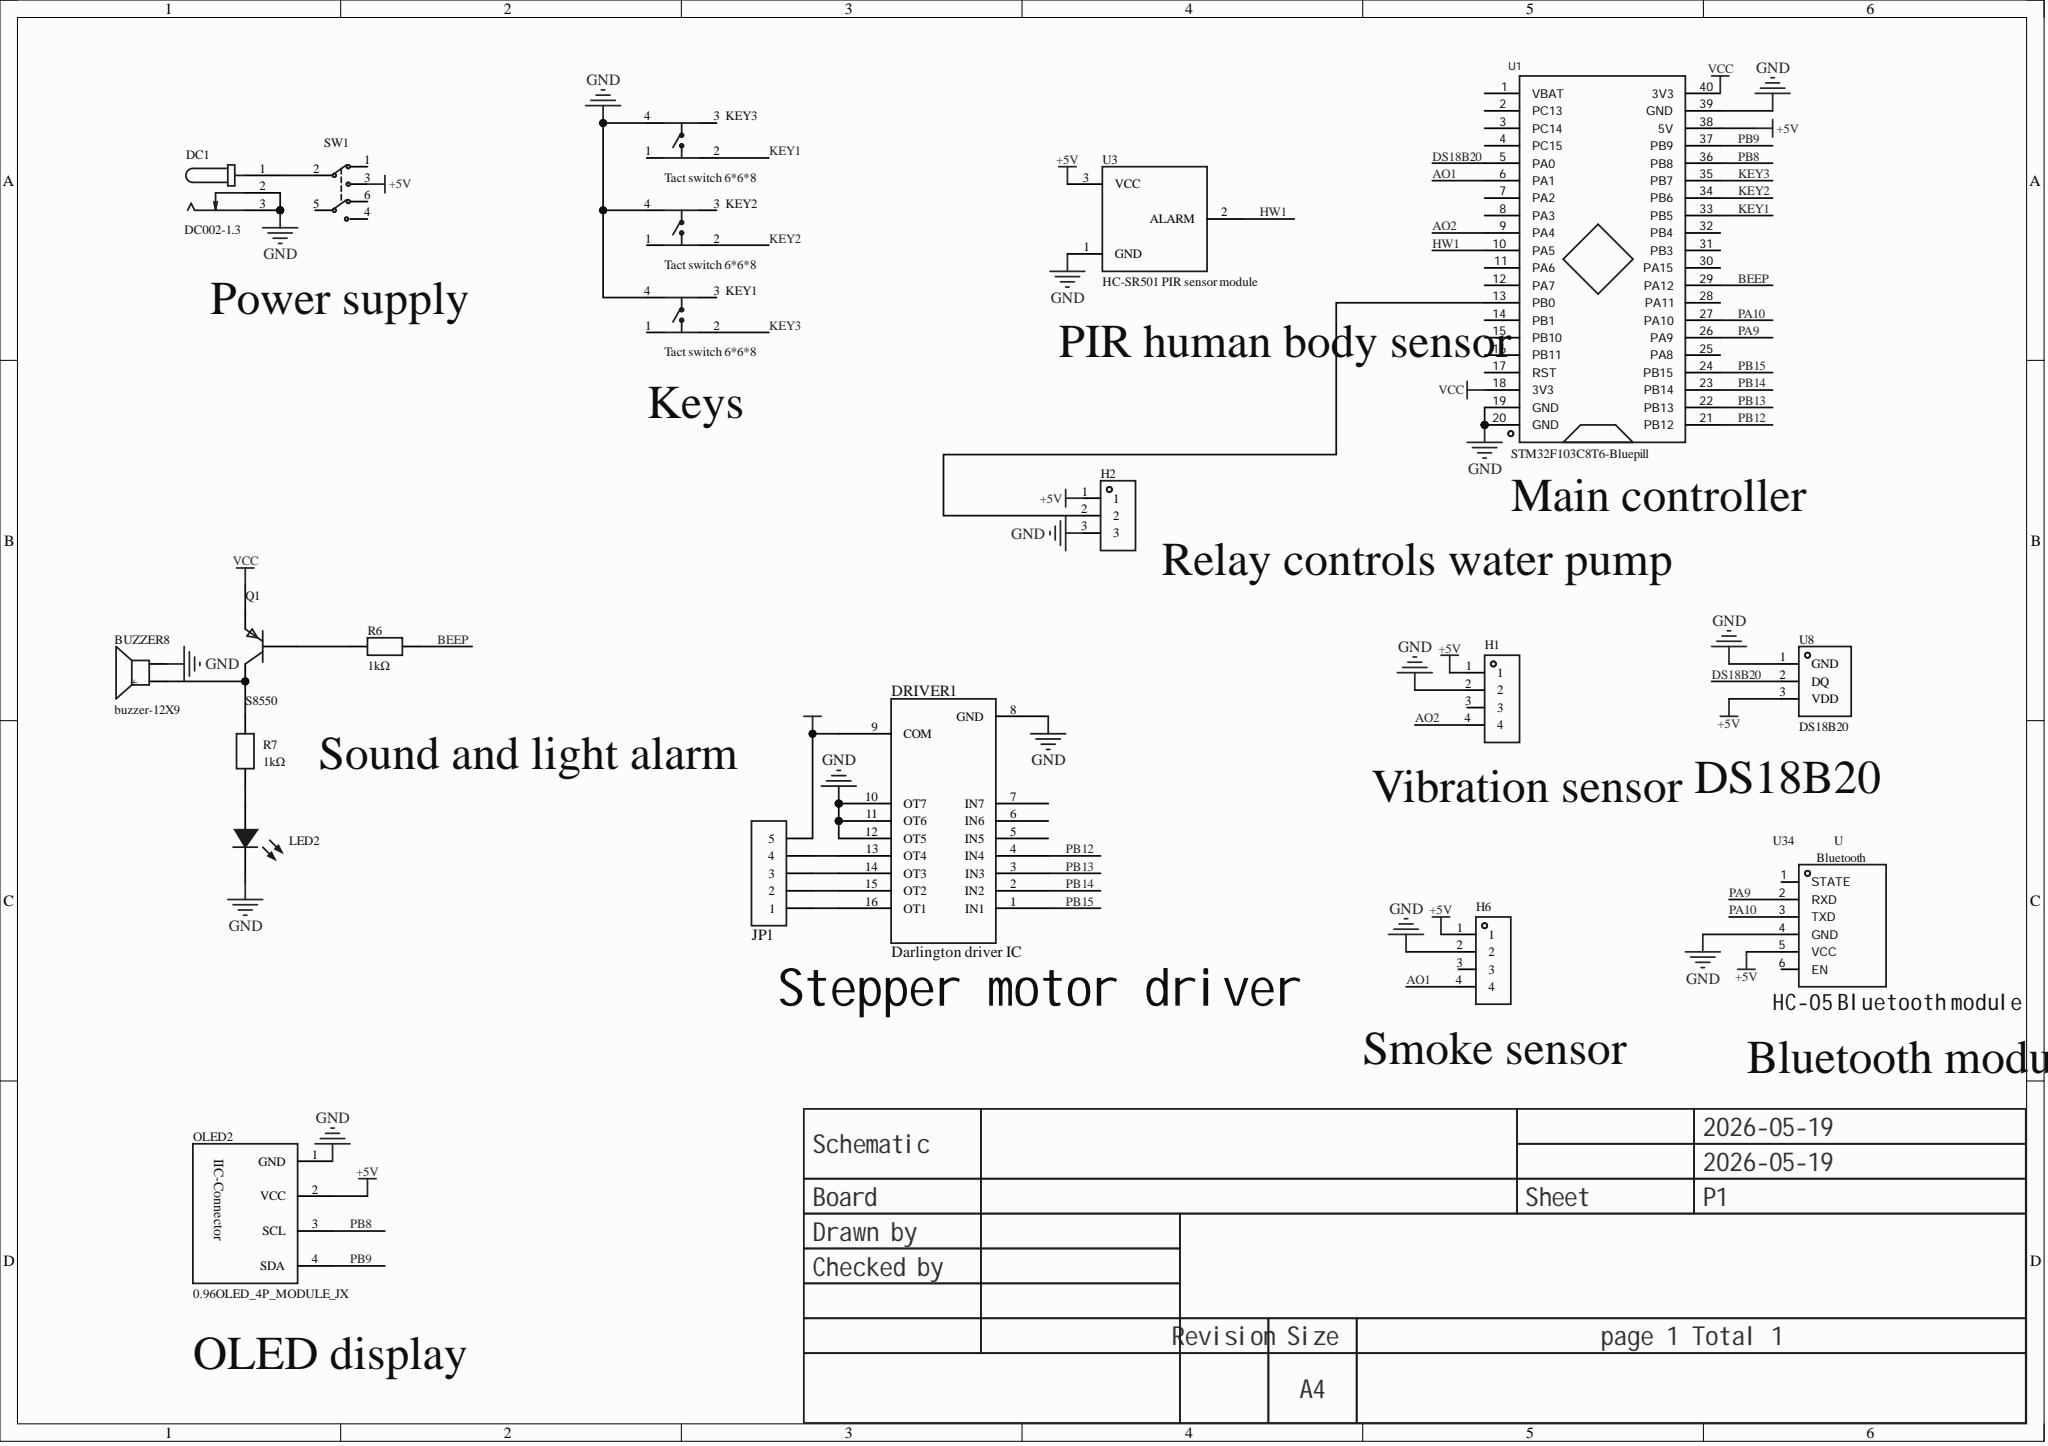Circuit board | Altium Designer | 20 parts | 28 nets
Bill of materials:
Comment,Description,Designator,Footprint,LibRef,Quantity
"buzzer-12X9","","BUZZER8","BUZ-TH_BD12.0-P7.60-D0.6-FD","buzzer-12X9","1"
"DC002-1.3","","DC1","DC-IN-TH_DC002-1.3","DC002-1.3","1"
"Darlington driver IC","","DRIVER1","DIP-16","达林顿驱动芯片","1"
"2.54-1*4P female","排数:单排;总孔位数:4;间距:2.54mm;插孔结构:1x4P;行距:-;安装类型:直插;圆孔/方孔:方孔;额定电流:3A;额定电压:-;插孔方向:顶部;塑高:-;触头材质:青铜;触头镀层:-;工作温度范围:-40℃~+105℃;焊接温度(最大值):-;","H1, H6","HDR-TH_4P-P2.54-V-F","2.54-1*4P母","2"
"","","H2","HDR-TH_3P-P2.54-V-F","HDR-F_2.54_1x3P","1"
"HDR-1X5","5P-?--","JP1","XH2.54-LI-5P","HDR-1X5","1"
"Tact switch 6*6*8","Circuit structure: SPST; contact rated current: -; button head type: Round Button; actuation direction: Top Actuated;","KEY1, KEY2, KEY3","KEY-TH_4P-L6.0-W6.0-P4.50-LS7.5","按键开关6*6*8","3"
"","","LED2","LED_TH-3mm","LED_TH-B_3mm","1"
"0.96OLED_4P_MODULE_JX","","OLED2","0.96OLED_4P","0.96OLED_4P_MODULE_JX","1"
"S8550","","Q1","TO-92-3_L4.5-W3.5-P1.27-L","S8550_C2931493","1"
"","Resistor type: metal film resistor; resistance: 1kΩ; tolerance: ±1%; power: 500mWS; temperature coefficient: ±50ppm/?; operating temperature range: -;","R6, R7","RES-TH_BD2.3-L6.5-P10.50-D0.5","插件电阻","2"
"","","SW1","自锁开关8.5*8.5","自锁开关","1"
"STM32F103C8T6-Bluepill","","U1","STM32F103C8T6-BLUEPILL","STM32F103C8T6-Bluepill","1"
"HC-SR501 PIR sensor module","","U3","HC-SR501","HC-SR501红外热释电模块","1"
"DS18B20","Temperature range: -55℃~+125℃; accuracy: ±0.4℃; interface type: -;","U8","TO-92-3_L4.9-W3.7-P1.27-L","DS18B20","1"
"","","U34","蓝牙level","蓝牙","1"
Netlist (Protel format):
[
BUZZER8
BUZ-TH_BD12.0-P7.60-D0.6-FD
buzzer-12X9



]
[
DC1
DC-IN-TH_DC002-1.3
DC002-1.3



]
[
DRIVER1
DIP-16
Darlington driver IC



]
[
H1
HDR-TH_4P-P2.54-V-F
2.54-1*4P female



]
[
H2
HDR-TH_3P-P2.54-V-F




]
[
H6
HDR-TH_4P-P2.54-V-F
2.54-1*4P female



]
[
JP1
XH2.54-LI-5P
HDR-1X5



]
[
KEY1
KEY-TH_4P-L6.0-W6.0-P4.50-LS7.5
Tact switch 6*6*8



]
[
KEY2
KEY-TH_4P-L6.0-W6.0-P4.50-LS7.5
Tact switch 6*6*8



]
[
KEY3
KEY-TH_4P-L6.0-W6.0-P4.50-LS7.5
Tact switch 6*6*8



]
[
LED2
LED_TH-3mm




]
[
OLED2
0.96OLED_4P
0.96OLED_4P_MODULE_JX



]
[
Q1
TO-92-3_L4.5-W3.5-P1.27-L
S8550



]
[
R6
RES-TH_BD2.3-L6.5-P10.50-D0.5




]
[
R7
RES-TH_BD2.3-L6.5-P10.50-D0.5




]
[
SW1
自锁开关8.5*8.5




]
[
U1
STM32F103C8T6-BLUEPILL
STM32F103C8T6-Bluepill



]
[
U3
HC-SR501
HC-SR501 PIR sensor module



]
[
U8
TO-92-3_L4.9-W3.7-P1.27-L
DS18B20



]
[
U34
蓝牙level




]
(
VCC
Q1-1
U1-18
U1-40
)
(
PB15
DRIVER1-1
U1-24
)
(
PB14
DRIVER1-2
U1-23
)
(
PB13
DRIVER1-3
U1-22
)
(
PB12
DRIVER1-4
U1-21
)
(
PB9
OLED2-4
U1-37
)
(
PB8
OLED2-3
U1-36
)
(
PA10
U1-27
U34-3
)
(
PA9
U1-26
U34-2
)
(
NetQ1_2
Q1-2
R6-1
)
(
NetLED2_1
LED2-1
R7-1
)
(
NetH2_2
H2-2
U1-13
)
(
NetDRIVER1_16
DRIVER1-16
JP1-1
)
(
NetDRIVER1_15
DRIVER1-15
JP1-2
)
(
NetDRIVER1_14
DRIVER1-14
JP1-3
)
(
NetDRIVER1_13
DRIVER1-13
JP1-4
)
(
NetDC1_1
DC1-1
SW1-2
)
(
NetBUZZER8_1
BUZZER8-1
Q1-3
R7-2
)
(
KEY3
KEY1-2
U1-35
)
(
KEY2
KEY2-2
U1-34
)
(
KEY1
KEY3-2
U1-33
)
(
HW1
U1-10
U3-2
)
(
GND
BUZZER8-2
DC1-2
DC1-3
DRIVER1-8
DRIVER1-10
DRIVER1-11
DRIVER1-12
H1-2
H2-3
H6-2
KEY1-4
KEY2-4
KEY3-4
LED2-2
OLED2-1
U1-19
U1-20
U1-39
U3-1
U8-1
U34-4
)
(
DS18B20
U1-5
U8-2
)
(
BEEP
R6-2
U1-29
)
(
AO2
H1-4
U1-9
)
(
AO1
H6-4
U1-6
)
(
+5V
DRIVER1-9
H1-1
H2-1
H6-1
JP1-5
OLED2-2
SW1-3
U1-38
U3-3
U8-3
U34-5
)